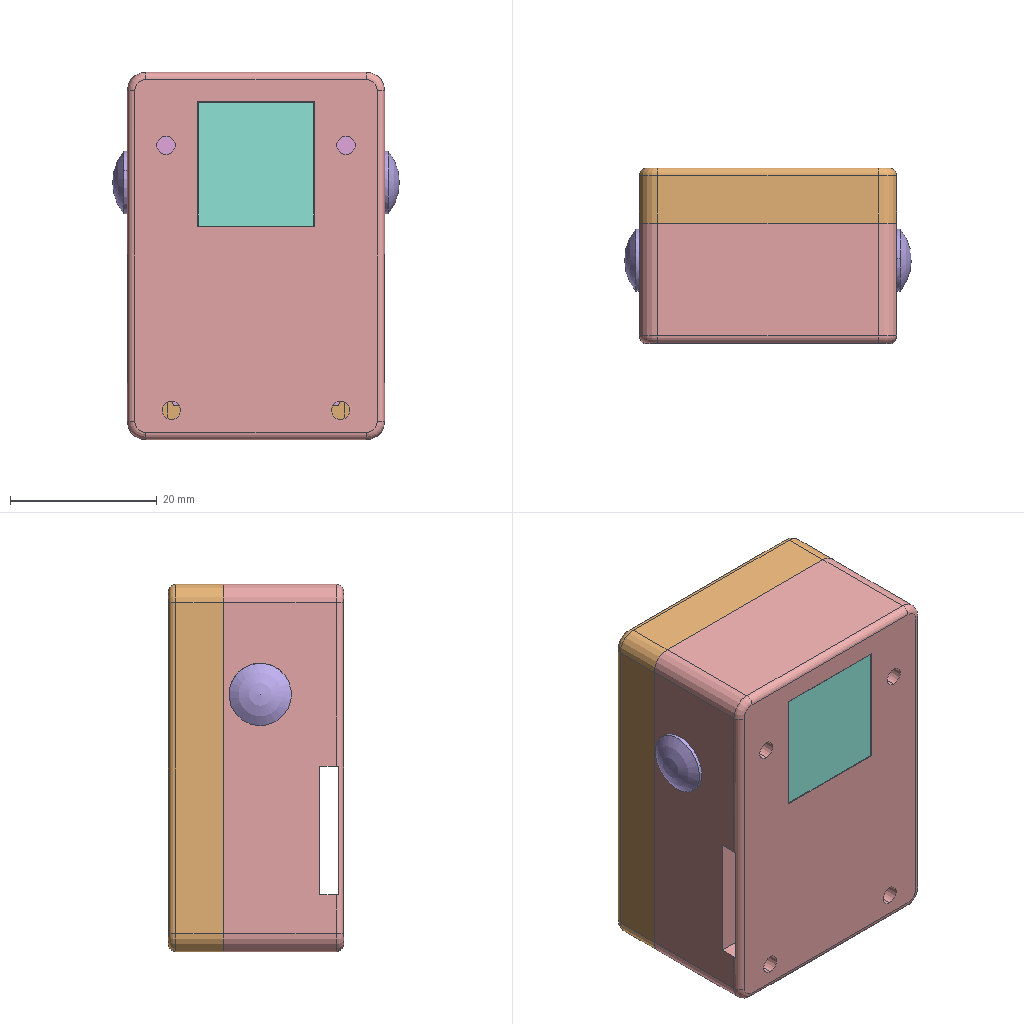Assembly | SolidWorks | 7 different items | 8 placed | box 39 x 24 x 50 mm
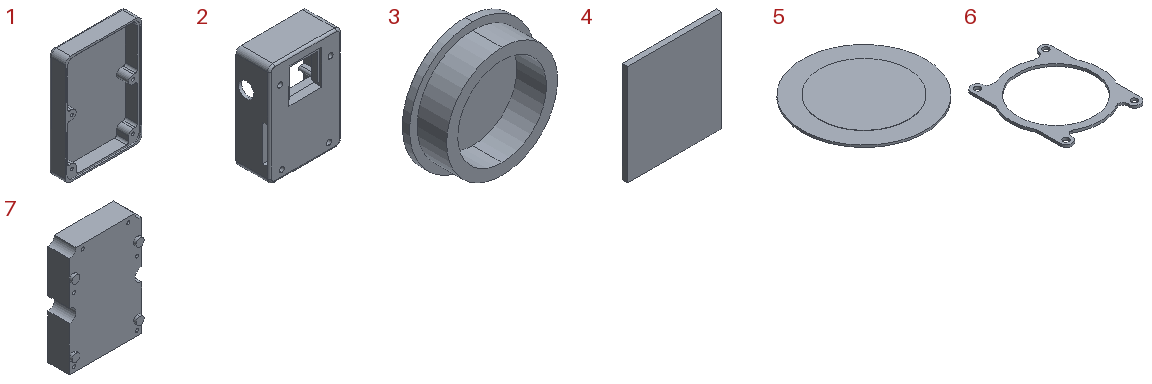Parts list (item | quantity | size | volume | features):
1 | x1 | 35 x 7.5 x 50 mm | 4265 mm3 | features ICE 5, Fillet 2, Extrusion 1, Scale 1
2 | x1 | 35 x 16.85 x 50 mm | 10296 mm3 | features ICE 14, Fillet 3, MoveFace 2, Extrusion 1, HoleWzd 1, Scale 1
3 | x2 | 8.5 x 4 x 8.5 mm | 104.507 mm3 | features ICE 2, Dome 1, Extrusion 1, Scale 1
4 | x1 | 15.76 x 0.95 x 16.86 mm | 252.428 mm3 | features Extrusion 1, Scale 1
5 | x1 | 17.5 x 17.5 x 0.35 mm | 78.294 mm3 | features BaseBody 1, Scale 1
6 | x1 | 17.8 x 19.9 x 0.5 mm | 54.481 mm3 | features BaseBody 1, Scale 1
7 | x1 | 27.5 x 9.25 x 40.9 mm | 9008 mm3 | features Extrusion 1, ICE 1, Scale 1
Mates (type | each side: item.copy, entity, surface, feature):
Coincident | 2.1 face plane Cut-Extrude2 | 5.1 face plane Imported1
Concentric | 2.1 face cylinder Cut-Extrude2 | 5.1 face cylinder Imported1
Coincident | 2.1 face plane Cut-Extrude1 | 6.1 face plane Imported1
Concentric | 2.1 face cylinder M2 Tapped Hole1 | 6.1 face cylinder Imported1 | 2 times
Concentric | 2.1 face cylinder Boss-Extrude2 | 7.1 face cylinder Boss-Extrude1 | 2 times
Coincident | 2.1 face plane Boss-Extrude2 | 7.1 face plane Boss-Extrude1
Coincident | 2.1 face plane Cut-Extrude10 | 4.1 face plane Boss-Extrude1
Parallel | 2.1 face plane Cut-Extrude10 | 4.1 face plane Boss-Extrude1 | 2 times
Coincident | 2.1 face plane Boss-Extrude1 | 1.1 face plane Boss-Extrude1
Concentric | 2.1 face cylinder Boss-Extrude3 | 1.1 face cylinder Cut-Extrude4 | 2 times
Concentric | 2.1 face cylinder Cut-Extrude14 | 3.1 face cylinder Boss-Extrude1
Coincident | 2.1 face plane Boss-Extrude1 | 3.1 face plane Boss-Extrude2
Concentric | 2.1 face cylinder Cut-Extrude14 | 3.2 face cylinder Boss-Extrude1
Coincident | 2.1 face plane Boss-Extrude1 | 3.2 face plane Boss-Extrude2
DistanceDim | 2.1 face plane Cut-Extrude10 | 4.1 face plane Boss-Extrude1 | 2 times